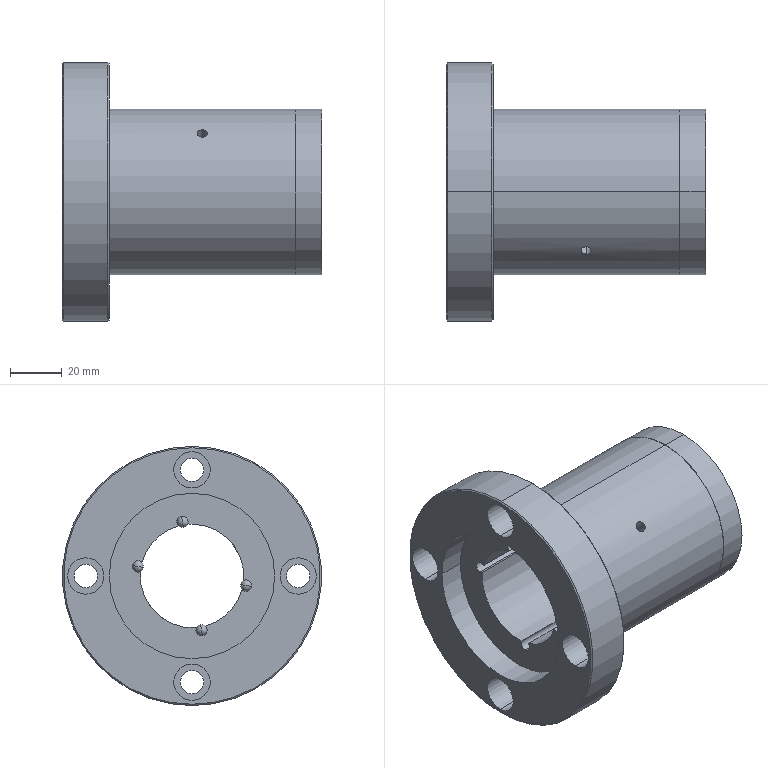Part | SolidWorks | features RevCut 6, Revolution 5, RefAxis 3, ICE 2, 3DProfileFeature 1, LockFeature 1 | 1 solid | 95 faces | box 100 x 100 x 100 mm | volume 246930 mm3 | cylinder 42 | sphere 40 | plane 9 | cone 4 | commonest cylinder face diameters 4.38 x9 9 x8 14 x8 40 x5 4 x4 63.8 x4